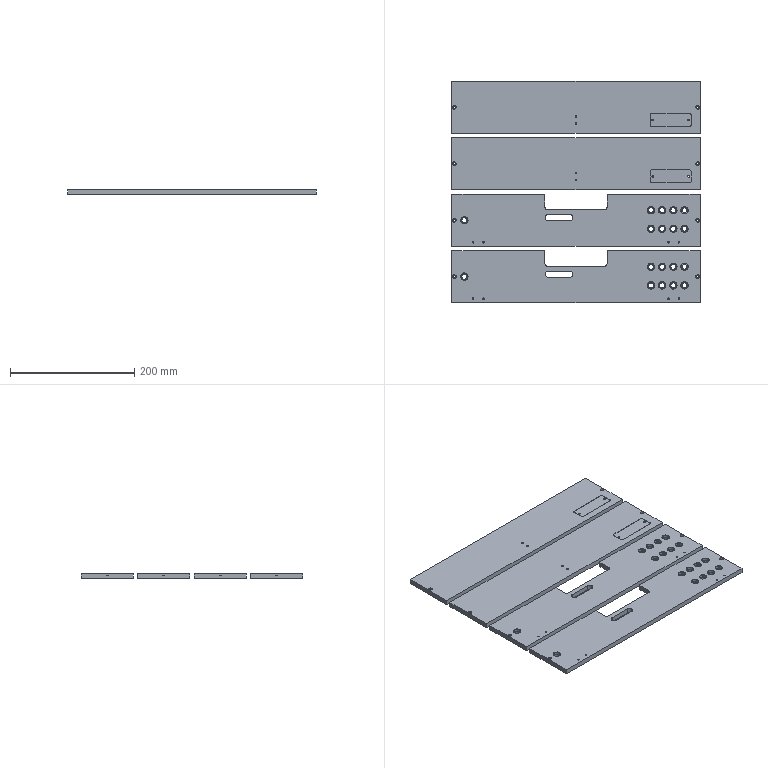Part | 4 solids | 296 faces | box 400 x 357 x 8 mm | volume 1014012 mm3 | cylinder 174 | plane 74 | cone 48 | commonest cylinder face diameters 2.5 x48 8.1 x36 11 x36 3.5 x16 6 x16 5 x8